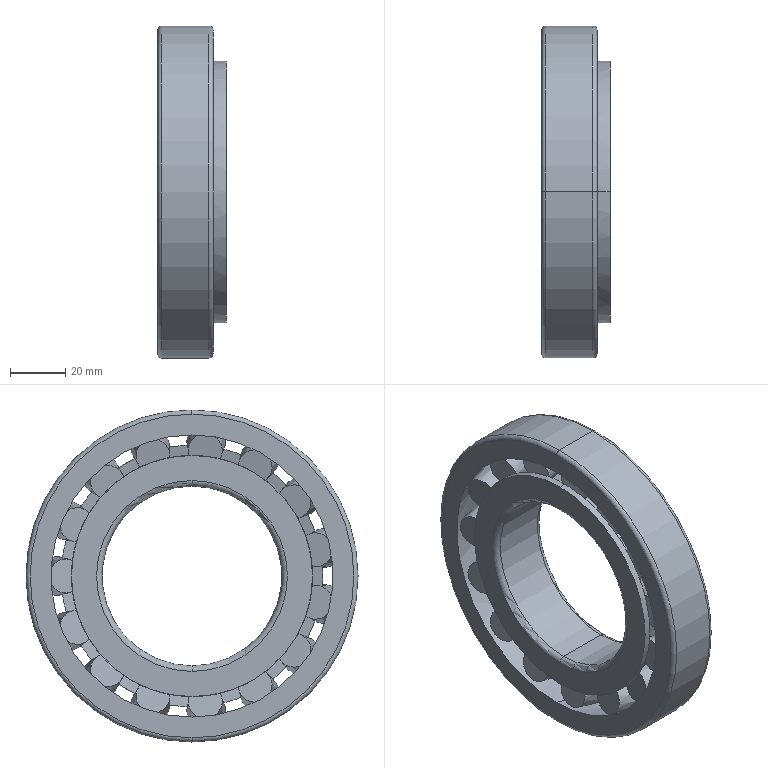Part | SolidWorks | features BaseBody 1 | 1 solid | 130 faces | box 24.75 x 120 x 120 mm | volume 131163 mm3 | cone 80 | plane 34 | torus 8 | cylinder 8 | commonest cylinder face diameters 65 x2 87.16 x2 94.547 x2 120 x2